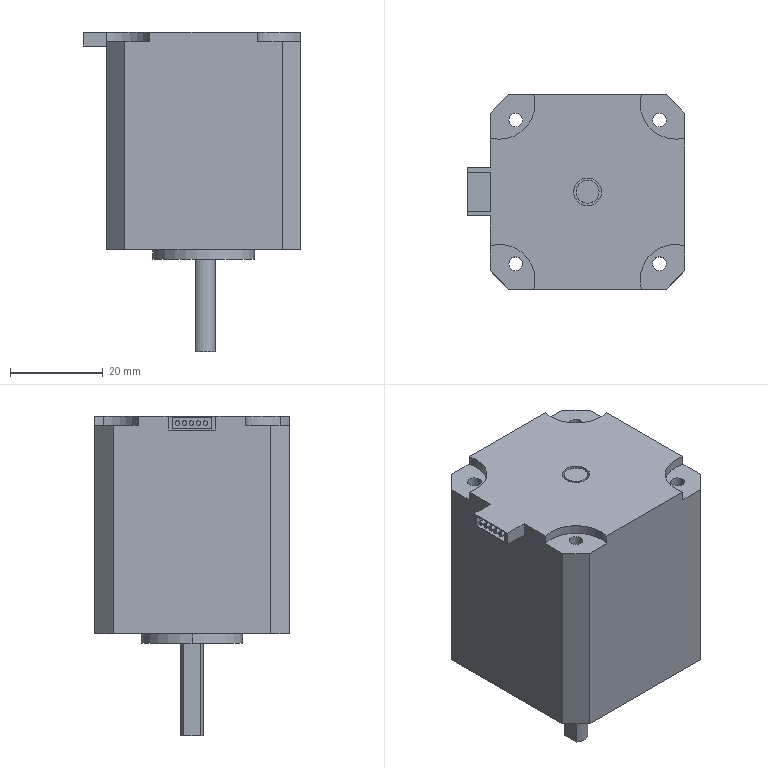Part | SolidWorks | features ICE 8, Extrusion 1 | 1 solid | 65 faces | box 47 x 42 x 69 mm | volume 80717 mm3 | plane 33 | cylinder 32 | commonest cylinder face diameters 1 x10 3 x8 15.282 x6 5 x4 6 x2 22 x2